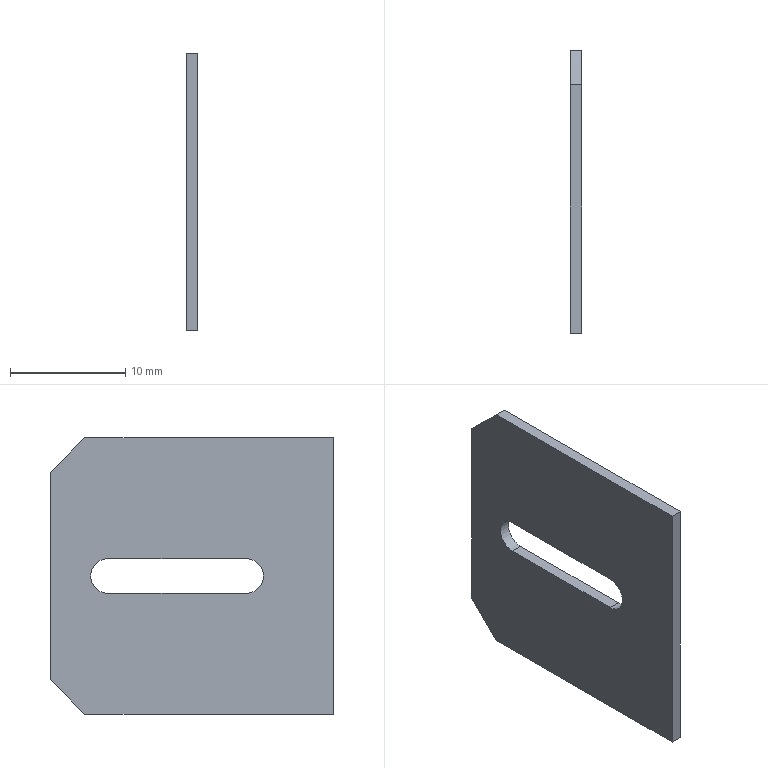Part | STEP file | ASND-0110-SDS_3_1 | 1 solid | 12 faces | box 1 x 24.6 x 24 mm | volume 538.331 mm3 | plane 10 | cylinder 2 | commonest cylinder face diameters 3 x2
STEP:
#1=CARTESIAN_POINT('',(0.,0.,0.));
#2=DIRECTION('',(0.,0.,1.));
#3=DIRECTION('',(1.,0.,0.));
#4=AXIS2_PLACEMENT_3D('',#1,#2,#3);
#5=CARTESIAN_POINT('',(-180.,82.3,67.4));
#6=VERTEX_POINT('',#5);
#7=CARTESIAN_POINT('',(-180.,79.3,70.4));
#8=VERTEX_POINT('',#7);
#9=CARTESIAN_POINT('',(-180.,82.3,67.4));
#10=DIRECTION('',(0.,-0.7071,0.7071));
#11=VECTOR('',#10,1.);
#12=LINE('',#9,#11);
#13=CARTESIAN_POINT('',(-180.5,80.8,68.9));
#14=DIRECTION('',(0.,0.7071,0.7071));
#15=DIRECTION('',(0.5774,-0.5774,0.5774));
#16=AXIS2_PLACEMENT_3D('',#13,#14,#15);
#17=PLANE('',#16);
#18=CARTESIAN_POINT('',(-1.443,1.633));
#19=DIRECTION('',(0.8165,-0.5774));
#20=VECTOR('',#19,1.);
#21=LINE('',#18,#20);
#22=(GEOMETRIC_REPRESENTATION_CONTEXT(2)PARAMETRIC_REPRESENTATION_CONTEXT()REPRESENTATION_CONTEXT('',''));
#23=DEFINITIONAL_REPRESENTATION('',(#21),#22);
#24=PCURVE('',#17,#23);
#25=CARTESIAN_POINT('',(-180.,0.,0.));
#26=DIRECTION('',(-1.,0.,0.));
#27=DIRECTION('',(0.,0.7071,0.7071));
#28=AXIS2_PLACEMENT_3D('',#25,#26,#27);
#29=PLANE('',#28);
#30=CARTESIAN_POINT('',(105.854,10.536));
#31=DIRECTION('',(0.,-1.));
#32=VECTOR('',#31,1.);
#33=LINE('',#30,#32);
#34=(GEOMETRIC_REPRESENTATION_CONTEXT(2)PARAMETRIC_REPRESENTATION_CONTEXT()REPRESENTATION_CONTEXT('',''));
#35=DEFINITIONAL_REPRESENTATION('',(#33),#34);
#36=PCURVE('',#29,#35);
#37=SURFACE_CURVE('',#12,(#24,#36),.PCURVE_S1.);
#38=EDGE_CURVE('',#6,#8,#37,.T.);
#39=ORIENTED_EDGE('',*,*,#38,.F.);
#40=CARTESIAN_POINT('',(-181.,82.3,67.4));
#41=VERTEX_POINT('',#40);
#42=CARTESIAN_POINT('',(-181.,82.3,67.4));
#43=DIRECTION('',(1.,0.,0.));
#44=VECTOR('',#43,1.);
#45=LINE('',#42,#44);
#46=CARTESIAN_POINT('',(-2.021,0.8165));
#47=DIRECTION('',(0.5774,0.8165));
#48=VECTOR('',#47,1.);
#49=LINE('',#46,#48);
#50=(GEOMETRIC_REPRESENTATION_CONTEXT(2)PARAMETRIC_REPRESENTATION_CONTEXT()REPRESENTATION_CONTEXT('',''));
#51=DEFINITIONAL_REPRESENTATION('',(#49),#50);
#52=PCURVE('',#17,#51);
#53=CARTESIAN_POINT('',(-181.,82.3,70.4));
#54=DIRECTION('',(0.,1.,0.));
#55=DIRECTION('',(0.7071,0.,0.7071));
#56=AXIS2_PLACEMENT_3D('',#53,#54,#55);
#57=PLANE('',#56);
#58=CARTESIAN_POINT('',(-2.121,2.121));
#59=DIRECTION('',(0.7071,0.7071));
#60=VECTOR('',#59,1.);
#61=LINE('',#58,#60);
#62=(GEOMETRIC_REPRESENTATION_CONTEXT(2)PARAMETRIC_REPRESENTATION_CONTEXT()REPRESENTATION_CONTEXT('',''));
#63=DEFINITIONAL_REPRESENTATION('',(#61),#62);
#64=PCURVE('',#57,#63);
#65=SURFACE_CURVE('',#45,(#52,#64),.PCURVE_S1.);
#66=EDGE_CURVE('',#41,#6,#65,.T.);
#67=ORIENTED_EDGE('',*,*,#66,.F.);
#68=CARTESIAN_POINT('',(-181.,79.3,70.4));
#69=VERTEX_POINT('',#68);
#70=CARTESIAN_POINT('',(-181.,79.3,70.4));
#71=DIRECTION('',(0.,0.7071,-0.7071));
#72=VECTOR('',#71,1.);
#73=LINE('',#70,#72);
#74=CARTESIAN_POINT('',(1.443,-1.633));
#75=DIRECTION('',(-0.8165,0.5774));
#76=VECTOR('',#75,1.);
#77=LINE('',#74,#76);
#78=(GEOMETRIC_REPRESENTATION_CONTEXT(2)PARAMETRIC_REPRESENTATION_CONTEXT()REPRESENTATION_CONTEXT('',''));
#79=DEFINITIONAL_REPRESENTATION('',(#77),#78);
#80=PCURVE('',#17,#79);
#81=CARTESIAN_POINT('',(-181.,0.,0.));
#82=DIRECTION('',(-1.,0.,0.));
#83=DIRECTION('',(0.,0.7071,0.7071));
#84=AXIS2_PLACEMENT_3D('',#81,#82,#83);
#85=PLANE('',#84);
#86=CARTESIAN_POINT('',(105.854,6.293));
#87=DIRECTION('',(0.,1.));
#88=VECTOR('',#87,1.);
#89=LINE('',#86,#88);
#90=(GEOMETRIC_REPRESENTATION_CONTEXT(2)PARAMETRIC_REPRESENTATION_CONTEXT()REPRESENTATION_CONTEXT('',''));
#91=DEFINITIONAL_REPRESENTATION('',(#89),#90);
#92=PCURVE('',#85,#91);
#93=SURFACE_CURVE('',#73,(#80,#92),.PCURVE_S1.);
#94=EDGE_CURVE('',#69,#41,#93,.T.);
#95=ORIENTED_EDGE('',*,*,#94,.F.);
#96=CARTESIAN_POINT('',(-181.,79.3,70.4));
#97=DIRECTION('',(1.,0.,0.));
#98=VECTOR('',#97,1.);
#99=LINE('',#96,#98);
#100=CARTESIAN_POINT('',(1.443,-1.633));
#101=DIRECTION('',(0.5774,0.8165));
#102=VECTOR('',#101,1.);
#103=LINE('',#100,#102);
#104=(GEOMETRIC_REPRESENTATION_CONTEXT(2)PARAMETRIC_REPRESENTATION_CONTEXT()REPRESENTATION_CONTEXT('',''));
#105=DEFINITIONAL_REPRESENTATION('',(#103),#104);
#106=PCURVE('',#17,#105);
#107=CARTESIAN_POINT('',(-181.,57.7,70.4));
#108=DIRECTION('',(0.,0.,1.));
#109=DIRECTION('',(0.7071,0.7071,0.));
#110=AXIS2_PLACEMENT_3D('',#107,#108,#109);
#111=PLANE('',#110);
#112=CARTESIAN_POINT('',(15.274,15.274));
#113=DIRECTION('',(0.7071,-0.7071));
#114=VECTOR('',#113,1.);
#115=LINE('',#112,#114);
#116=(GEOMETRIC_REPRESENTATION_CONTEXT(2)PARAMETRIC_REPRESENTATION_CONTEXT()REPRESENTATION_CONTEXT('',''));
#117=DEFINITIONAL_REPRESENTATION('',(#115),#116);
#118=PCURVE('',#111,#117);
#119=SURFACE_CURVE('',#99,(#106,#118),.PCURVE_S1.);
#120=EDGE_CURVE('',#69,#8,#119,.T.);
#121=ORIENTED_EDGE('',*,*,#120,.T.);
#122=EDGE_LOOP('',(#39,#67,#95,#121));
#123=FACE_BOUND('',#122,.T.);
#124=ADVANCED_FACE('',(#123),#17,.T.);
#125=CARTESIAN_POINT('',(-180.,79.3,46.4));
#126=VERTEX_POINT('',#125);
#127=CARTESIAN_POINT('',(-180.,82.3,49.4));
#128=VERTEX_POINT('',#127);
#129=CARTESIAN_POINT('',(-180.,79.3,46.4));
#130=DIRECTION('',(0.,0.7071,0.7071));
#131=VECTOR('',#130,1.);
#132=LINE('',#129,#131);
#133=CARTESIAN_POINT('',(88.883,23.264));
#134=DIRECTION('',(1.,0.));
#135=VECTOR('',#134,1.);
#136=LINE('',#133,#135);
#137=(GEOMETRIC_REPRESENTATION_CONTEXT(2)PARAMETRIC_REPRESENTATION_CONTEXT()REPRESENTATION_CONTEXT('',''));
#138=DEFINITIONAL_REPRESENTATION('',(#136),#137);
#139=PCURVE('',#29,#138);
#140=CARTESIAN_POINT('',(-180.5,80.8,47.9));
#141=DIRECTION('',(0.,0.7071,-0.7071));
#142=DIRECTION('',(0.5774,0.5774,0.5774));
#143=AXIS2_PLACEMENT_3D('',#140,#141,#142);
#144=PLANE('',#143);
#145=CARTESIAN_POINT('',(-1.443,1.633));
#146=DIRECTION('',(0.8165,-0.5774));
#147=VECTOR('',#146,1.);
#148=LINE('',#145,#147);
#149=(GEOMETRIC_REPRESENTATION_CONTEXT(2)PARAMETRIC_REPRESENTATION_CONTEXT()REPRESENTATION_CONTEXT('',''));
#150=DEFINITIONAL_REPRESENTATION('',(#148),#149);
#151=PCURVE('',#144,#150);
#152=SURFACE_CURVE('',#132,(#139,#151),.PCURVE_S1.);
#153=EDGE_CURVE('',#126,#128,#152,.T.);
#154=ORIENTED_EDGE('',*,*,#153,.T.);
#155=CARTESIAN_POINT('',(-180.,82.3,67.4));
#156=DIRECTION('',(0.,0.,-1.));
#157=VECTOR('',#156,1.);
#158=LINE('',#155,#157);
#159=CARTESIAN_POINT('',(105.854,10.536));
#160=DIRECTION('',(-0.7071,0.7071));
#161=VECTOR('',#160,1.);
#162=LINE('',#159,#161);
#163=(GEOMETRIC_REPRESENTATION_CONTEXT(2)PARAMETRIC_REPRESENTATION_CONTEXT()REPRESENTATION_CONTEXT('',''));
#164=DEFINITIONAL_REPRESENTATION('',(#162),#163);
#165=PCURVE('',#29,#164);
#166=CARTESIAN_POINT('',(-1.414,2.828));
#167=DIRECTION('',(-0.7071,0.7071));
#168=VECTOR('',#167,1.);
#169=LINE('',#166,#168);
#170=(GEOMETRIC_REPRESENTATION_CONTEXT(2)PARAMETRIC_REPRESENTATION_CONTEXT()REPRESENTATION_CONTEXT('',''));
#171=DEFINITIONAL_REPRESENTATION('',(#169),#170);
#172=PCURVE('',#57,#171);
#173=SURFACE_CURVE('',#158,(#165,#172),.PCURVE_S1.);
#174=EDGE_CURVE('',#6,#128,#173,.T.);
#175=ORIENTED_EDGE('',*,*,#174,.F.);
#176=ORIENTED_EDGE('',*,*,#38,.T.);
#177=CARTESIAN_POINT('',(-180.,57.7,70.4));
#178=VERTEX_POINT('',#177);
#179=CARTESIAN_POINT('',(-180.,57.7,70.4));
#180=DIRECTION('',(0.,1.,0.));
#181=VECTOR('',#180,1.);
#182=LINE('',#179,#181);
#183=CARTESIAN_POINT('',(90.58,-8.98));
#184=DIRECTION('',(0.7071,0.7071));
#185=VECTOR('',#184,1.);
#186=LINE('',#183,#185);
#187=(GEOMETRIC_REPRESENTATION_CONTEXT(2)PARAMETRIC_REPRESENTATION_CONTEXT()REPRESENTATION_CONTEXT('',''));
#188=DEFINITIONAL_REPRESENTATION('',(#186),#187);
#189=PCURVE('',#29,#188);
#190=CARTESIAN_POINT('',(0.7071,-0.7071));
#191=DIRECTION('',(0.7071,0.7071));
#192=VECTOR('',#191,1.);
#193=LINE('',#190,#192);
#194=(GEOMETRIC_REPRESENTATION_CONTEXT(2)PARAMETRIC_REPRESENTATION_CONTEXT()REPRESENTATION_CONTEXT('',''));
#195=DEFINITIONAL_REPRESENTATION('',(#193),#194);
#196=PCURVE('',#111,#195);
#197=SURFACE_CURVE('',#182,(#189,#196),.PCURVE_S1.);
#198=EDGE_CURVE('',#178,#8,#197,.T.);
#199=ORIENTED_EDGE('',*,*,#198,.F.);
#200=CARTESIAN_POINT('',(-180.,57.7,46.4));
#201=VERTEX_POINT('',#200);
#202=CARTESIAN_POINT('',(-180.,57.7,46.4));
#203=DIRECTION('',(0.,0.,1.));
#204=VECTOR('',#203,1.);
#205=LINE('',#202,#204);
#206=CARTESIAN_POINT('',(73.61,7.99));
#207=DIRECTION('',(0.7071,-0.7071));
#208=VECTOR('',#207,1.);
#209=LINE('',#206,#208);
#210=(GEOMETRIC_REPRESENTATION_CONTEXT(2)PARAMETRIC_REPRESENTATION_CONTEXT()REPRESENTATION_CONTEXT('',''));
#211=DEFINITIONAL_REPRESENTATION('',(#209),#210);
#212=PCURVE('',#29,#211);
#213=CARTESIAN_POINT('',(-181.,57.7,46.4));
#214=DIRECTION('',(0.,-1.,0.));
#215=DIRECTION('',(0.7071,0.,0.7071));
#216=AXIS2_PLACEMENT_3D('',#213,#214,#215);
#217=PLANE('',#216);
#218=CARTESIAN_POINT('',(0.7071,-0.7071));
#219=DIRECTION('',(0.7071,0.7071));
#220=VECTOR('',#219,1.);
#221=LINE('',#218,#220);
#222=(GEOMETRIC_REPRESENTATION_CONTEXT(2)PARAMETRIC_REPRESENTATION_CONTEXT()REPRESENTATION_CONTEXT('',''));
#223=DEFINITIONAL_REPRESENTATION('',(#221),#222);
#224=PCURVE('',#217,#223);
#225=SURFACE_CURVE('',#205,(#212,#224),.PCURVE_S1.);
#226=EDGE_CURVE('',#201,#178,#225,.T.);
#227=ORIENTED_EDGE('',*,*,#226,.F.);
#228=CARTESIAN_POINT('',(-180.,79.3,46.4));
#229=DIRECTION('',(0.,-1.,0.));
#230=VECTOR('',#229,1.);
#231=LINE('',#228,#230);
#232=CARTESIAN_POINT('',(88.883,23.264));
#233=DIRECTION('',(-0.7071,-0.7071));
#234=VECTOR('',#233,1.);
#235=LINE('',#232,#234);
#236=(GEOMETRIC_REPRESENTATION_CONTEXT(2)PARAMETRIC_REPRESENTATION_CONTEXT()REPRESENTATION_CONTEXT('',''));
#237=DEFINITIONAL_REPRESENTATION('',(#235),#236);
#238=PCURVE('',#29,#237);
#239=CARTESIAN_POINT('',(-181.,82.3,46.4));
#240=DIRECTION('',(0.,0.,-1.));
#241=DIRECTION('',(0.7071,0.7071,0.));
#242=AXIS2_PLACEMENT_3D('',#239,#240,#241);
#243=PLANE('',#242);
#244=CARTESIAN_POINT('',(-1.414,2.828));
#245=DIRECTION('',(-0.7071,0.7071));
#246=VECTOR('',#245,1.);
#247=LINE('',#244,#246);
#248=(GEOMETRIC_REPRESENTATION_CONTEXT(2)PARAMETRIC_REPRESENTATION_CONTEXT()REPRESENTATION_CONTEXT('',''));
#249=DEFINITIONAL_REPRESENTATION('',(#247),#248);
#250=PCURVE('',#243,#249);
#251=SURFACE_CURVE('',#231,(#238,#250),.PCURVE_S1.);
#252=EDGE_CURVE('',#126,#201,#251,.T.);
#253=ORIENTED_EDGE('',*,*,#252,.F.);
#254=EDGE_LOOP('',(#154,#175,#176,#199,#227,#253));
#255=FACE_BOUND('',#254,.T.);
#256=CARTESIAN_POINT('',(-180.,77.3,56.9));
#257=VERTEX_POINT('',#256);
#258=CARTESIAN_POINT('',(-180.,77.3,59.9));
#259=VERTEX_POINT('',#258);
#260=CARTESIAN_POINT('',(-180.,77.3,58.4));
#261=DIRECTION('',(1.,0.,0.));
#262=DIRECTION('',(0.,0.,-1.));
#263=AXIS2_PLACEMENT_3D('',#260,#261,#262);
#264=CIRCLE('',#263,1.5);
#265=CARTESIAN_POINT('',(94.894,14.425));
#266=CARTESIAN_POINT('',(96.731,16.262));
#267=CARTESIAN_POINT('',(97.403,13.753));
#268=CARTESIAN_POINT('',(98.076,11.243));
#269=CARTESIAN_POINT('',(95.566,11.915));
#270=CARTESIAN_POINT('',(93.057,12.588));
#271=CARTESIAN_POINT('',(94.894,14.425));
#272=(BOUNDED_CURVE()B_SPLINE_CURVE(2,(#265,#266,#267,#268,#269,#270,#271),.UNSPECIFIED.,.T.,.F.)B_SPLINE_CURVE_WITH_KNOTS((1,2,2,2,2,1),(-2.094,0.,2.094,4.189,6.283,8.378),.UNSPECIFIED.)CURVE()GEOMETRIC_REPRESENTATION_ITEM()RATIONAL_B_SPLINE_CURVE((1.,0.5,1.,0.5,1.,0.5,1.))REPRESENTATION_ITEM(''));
#273=(GEOMETRIC_REPRESENTATION_CONTEXT(2)PARAMETRIC_REPRESENTATION_CONTEXT()REPRESENTATION_CONTEXT('',''));
#274=DEFINITIONAL_REPRESENTATION('',(#272),#273);
#275=PCURVE('',#29,#274);
#276=CARTESIAN_POINT('',(-181.,77.3,58.4));
#277=DIRECTION('',(-1.,0.,0.));
#278=DIRECTION('',(0.,0.,1.));
#279=AXIS2_PLACEMENT_3D('',#276,#277,#278);
#280=CYLINDRICAL_SURFACE('',#279,1.5);
#281=CARTESIAN_POINT('',(3.142,-1.));
#282=DIRECTION('',(-1.,0.));
#283=VECTOR('',#282,1.);
#284=LINE('',#281,#283);
#285=(GEOMETRIC_REPRESENTATION_CONTEXT(2)PARAMETRIC_REPRESENTATION_CONTEXT()REPRESENTATION_CONTEXT('',''));
#286=DEFINITIONAL_REPRESENTATION('',(#284),#285);
#287=PCURVE('',#280,#286);
#288=SURFACE_CURVE('',#264,(#275,#287),.PCURVE_S1.);
#289=EDGE_CURVE('',#257,#259,#288,.T.);
#290=ORIENTED_EDGE('',*,*,#289,.F.);
#291=CARTESIAN_POINT('',(-180.,65.3,56.9));
#292=VERTEX_POINT('',#291);
#293=CARTESIAN_POINT('',(-180.,65.3,56.9));
#294=DIRECTION('',(0.,1.,0.));
#295=VECTOR('',#294,1.);
#296=LINE('',#293,#295);
#297=CARTESIAN_POINT('',(86.408,5.94));
#298=DIRECTION('',(0.7071,0.7071));
#299=VECTOR('',#298,1.);
#300=LINE('',#297,#299);
#301=(GEOMETRIC_REPRESENTATION_CONTEXT(2)PARAMETRIC_REPRESENTATION_CONTEXT()REPRESENTATION_CONTEXT('',''));
#302=DEFINITIONAL_REPRESENTATION('',(#300),#301);
#303=PCURVE('',#29,#302);
#304=CARTESIAN_POINT('',(-181.,65.3,56.9));
#305=DIRECTION('',(0.,0.,1.));
#306=DIRECTION('',(0.7071,0.7071,0.));
#307=AXIS2_PLACEMENT_3D('',#304,#305,#306);
#308=PLANE('',#307);
#309=CARTESIAN_POINT('',(0.7071,-0.7071));
#310=DIRECTION('',(0.7071,0.7071));
#311=VECTOR('',#310,1.);
#312=LINE('',#309,#311);
#313=(GEOMETRIC_REPRESENTATION_CONTEXT(2)PARAMETRIC_REPRESENTATION_CONTEXT()REPRESENTATION_CONTEXT('',''));
#314=DEFINITIONAL_REPRESENTATION('',(#312),#313);
#315=PCURVE('',#308,#314);
#316=SURFACE_CURVE('',#296,(#303,#315),.PCURVE_S1.);
#317=EDGE_CURVE('',#292,#257,#316,.T.);
#318=ORIENTED_EDGE('',*,*,#317,.F.);
#319=CARTESIAN_POINT('',(-180.,65.3,59.9));
#320=VERTEX_POINT('',#319);
#321=CARTESIAN_POINT('',(-180.,65.3,58.4));
#322=DIRECTION('',(1.,0.,0.));
#323=DIRECTION('',(0.,0.,1.));
#324=AXIS2_PLACEMENT_3D('',#321,#322,#323);
#325=CIRCLE('',#324,1.5);
#326=CARTESIAN_POINT('',(88.53,3.818));
#327=CARTESIAN_POINT('',(86.693,1.981));
#328=CARTESIAN_POINT('',(86.02,4.491));
#329=CARTESIAN_POINT('',(85.348,7.));
#330=CARTESIAN_POINT('',(87.857,6.328));
#331=CARTESIAN_POINT('',(90.367,5.655));
#332=CARTESIAN_POINT('',(88.53,3.818));
#333=(BOUNDED_CURVE()B_SPLINE_CURVE(2,(#326,#327,#328,#329,#330,#331,#332),.UNSPECIFIED.,.T.,.F.)B_SPLINE_CURVE_WITH_KNOTS((1,2,2,2,2,1),(-2.094,0.,2.094,4.189,6.283,8.378),.UNSPECIFIED.)CURVE()GEOMETRIC_REPRESENTATION_ITEM()RATIONAL_B_SPLINE_CURVE((1.,0.5,1.,0.5,1.,0.5,1.))REPRESENTATION_ITEM(''));
#334=(GEOMETRIC_REPRESENTATION_CONTEXT(2)PARAMETRIC_REPRESENTATION_CONTEXT()REPRESENTATION_CONTEXT('',''));
#335=DEFINITIONAL_REPRESENTATION('',(#333),#334);
#336=PCURVE('',#29,#335);
#337=CARTESIAN_POINT('',(-181.,65.3,58.4));
#338=DIRECTION('',(-1.,0.,0.));
#339=DIRECTION('',(0.,0.,1.));
#340=AXIS2_PLACEMENT_3D('',#337,#338,#339);
#341=CYLINDRICAL_SURFACE('',#340,1.5);
#342=CARTESIAN_POINT('',(6.283,-1.));
#343=DIRECTION('',(-1.,0.));
#344=VECTOR('',#343,1.);
#345=LINE('',#342,#344);
#346=(GEOMETRIC_REPRESENTATION_CONTEXT(2)PARAMETRIC_REPRESENTATION_CONTEXT()REPRESENTATION_CONTEXT('',''));
#347=DEFINITIONAL_REPRESENTATION('',(#345),#346);
#348=PCURVE('',#341,#347);
#349=SURFACE_CURVE('',#325,(#336,#348),.PCURVE_S1.);
#350=EDGE_CURVE('',#320,#292,#349,.T.);
#351=ORIENTED_EDGE('',*,*,#350,.F.);
#352=CARTESIAN_POINT('',(-180.,77.3,59.9));
#353=DIRECTION('',(0.,-1.,0.));
#354=VECTOR('',#353,1.);
#355=LINE('',#352,#354);
#356=CARTESIAN_POINT('',(97.015,12.304));
#357=DIRECTION('',(-0.7071,-0.7071));
#358=VECTOR('',#357,1.);
#359=LINE('',#356,#358);
#360=(GEOMETRIC_REPRESENTATION_CONTEXT(2)PARAMETRIC_REPRESENTATION_CONTEXT()REPRESENTATION_CONTEXT('',''));
#361=DEFINITIONAL_REPRESENTATION('',(#359),#360);
#362=PCURVE('',#29,#361);
#363=CARTESIAN_POINT('',(-181.,77.3,59.9));
#364=DIRECTION('',(0.,0.,-1.));
#365=DIRECTION('',(0.7071,0.7071,0.));
#366=AXIS2_PLACEMENT_3D('',#363,#364,#365);
#367=PLANE('',#366);
#368=CARTESIAN_POINT('',(0.7071,0.7071));
#369=DIRECTION('',(-0.7071,0.7071));
#370=VECTOR('',#369,1.);
#371=LINE('',#368,#370);
#372=(GEOMETRIC_REPRESENTATION_CONTEXT(2)PARAMETRIC_REPRESENTATION_CONTEXT()REPRESENTATION_CONTEXT('',''));
#373=DEFINITIONAL_REPRESENTATION('',(#371),#372);
#374=PCURVE('',#367,#373);
#375=SURFACE_CURVE('',#355,(#362,#374),.PCURVE_S1.);
#376=EDGE_CURVE('',#259,#320,#375,.T.);
#377=ORIENTED_EDGE('',*,*,#376,.F.);
#378=EDGE_LOOP('',(#290,#318,#351,#377));
#379=FACE_BOUND('',#378,.T.);
#380=ADVANCED_FACE('',(#255,#379),#29,.F.);
#381=CARTESIAN_POINT('',(-181.,77.3,59.9));
#382=VERTEX_POINT('',#381);
#383=CARTESIAN_POINT('',(-181.,77.3,59.9));
#384=DIRECTION('',(1.,0.,0.));
#385=VECTOR('',#384,1.);
#386=LINE('',#383,#385);
#387=CARTESIAN_POINT('',(0.,0.));
#388=DIRECTION('',(0.,-1.));
#389=VECTOR('',#388,1.);
#390=LINE('',#387,#389);
#391=(GEOMETRIC_REPRESENTATION_CONTEXT(2)PARAMETRIC_REPRESENTATION_CONTEXT()REPRESENTATION_CONTEXT('',''));
#392=DEFINITIONAL_REPRESENTATION('',(#390),#391);
#393=PCURVE('',#280,#392);
#394=CARTESIAN_POINT('',(0.,0.));
#395=DIRECTION('',(0.7071,0.7071));
#396=VECTOR('',#395,1.);
#397=LINE('',#394,#396);
#398=(GEOMETRIC_REPRESENTATION_CONTEXT(2)PARAMETRIC_REPRESENTATION_CONTEXT()REPRESENTATION_CONTEXT('',''));
#399=DEFINITIONAL_REPRESENTATION('',(#397),#398);
#400=PCURVE('',#367,#399);
#401=SURFACE_CURVE('',#386,(#393,#400),.PCURVE_S1.);
#402=EDGE_CURVE('',#382,#259,#401,.T.);
#403=ORIENTED_EDGE('',*,*,#402,.T.);
#404=ORIENTED_EDGE('',*,*,#289,.F.);
#405=CARTESIAN_POINT('',(-181.,77.3,56.9));
#406=VERTEX_POINT('',#405);
#407=CARTESIAN_POINT('',(-181.,77.3,56.9));
#408=DIRECTION('',(1.,0.,0.));
#409=VECTOR('',#408,1.);
#410=LINE('',#407,#409);
#411=CARTESIAN_POINT('',(3.142,0.));
#412=DIRECTION('',(0.,-1.));
#413=VECTOR('',#412,1.);
#414=LINE('',#411,#413);
#415=(GEOMETRIC_REPRESENTATION_CONTEXT(2)PARAMETRIC_REPRESENTATION_CONTEXT()REPRESENTATION_CONTEXT('',''));
#416=DEFINITIONAL_REPRESENTATION('',(#414),#415);
#417=PCURVE('',#280,#416);
#418=CARTESIAN_POINT('',(8.485,8.485));
#419=DIRECTION('',(0.7071,-0.7071));
#420=VECTOR('',#419,1.);
#421=LINE('',#418,#420);
#422=(GEOMETRIC_REPRESENTATION_CONTEXT(2)PARAMETRIC_REPRESENTATION_CONTEXT()REPRESENTATION_CONTEXT('',''));
#423=DEFINITIONAL_REPRESENTATION('',(#421),#422);
#424=PCURVE('',#308,#423);
#425=SURFACE_CURVE('',#410,(#417,#424),.PCURVE_S1.);
#426=EDGE_CURVE('',#406,#257,#425,.T.);
#427=ORIENTED_EDGE('',*,*,#426,.F.);
#428=CARTESIAN_POINT('',(-181.,77.3,58.4));
#429=DIRECTION('',(1.,0.,0.));
#430=DIRECTION('',(0.,0.,-1.));
#431=AXIS2_PLACEMENT_3D('',#428,#429,#430);
#432=CIRCLE('',#431,1.5);
#433=CARTESIAN_POINT('',(3.142,0.));
#434=DIRECTION('',(-1.,0.));
#435=VECTOR('',#434,1.);
#436=LINE('',#433,#435);
#437=(GEOMETRIC_REPRESENTATION_CONTEXT(2)PARAMETRIC_REPRESENTATION_CONTEXT()REPRESENTATION_CONTEXT('',''));
#438=DEFINITIONAL_REPRESENTATION('',(#436),#437);
#439=PCURVE('',#280,#438);
#440=CARTESIAN_POINT('',(94.894,14.425));
#441=CARTESIAN_POINT('',(96.731,16.262));
#442=CARTESIAN_POINT('',(97.403,13.753));
#443=CARTESIAN_POINT('',(98.076,11.243));
#444=CARTESIAN_POINT('',(95.566,11.915));
#445=CARTESIAN_POINT('',(93.057,12.588));
#446=CARTESIAN_POINT('',(94.894,14.425));
#447=(BOUNDED_CURVE()B_SPLINE_CURVE(2,(#440,#441,#442,#443,#444,#445,#446),.UNSPECIFIED.,.T.,.F.)B_SPLINE_CURVE_WITH_KNOTS((1,2,2,2,2,1),(-2.094,0.,2.094,4.189,6.283,8.378),.UNSPECIFIED.)CURVE()GEOMETRIC_REPRESENTATION_ITEM()RATIONAL_B_SPLINE_CURVE((1.,0.5,1.,0.5,1.,0.5,1.))REPRESENTATION_ITEM(''));
#448=(GEOMETRIC_REPRESENTATION_CONTEXT(2)PARAMETRIC_REPRESENTATION_CONTEXT()REPRESENTATION_CONTEXT('',''));
#449=DEFINITIONAL_REPRESENTATION('',(#447),#448);
#450=PCURVE('',#85,#449);
#451=SURFACE_CURVE('',#432,(#439,#450),.PCURVE_S1.);
#452=EDGE_CURVE('',#406,#382,#451,.T.);
#453=ORIENTED_EDGE('',*,*,#452,.T.);
#454=EDGE_LOOP('',(#403,#404,#427,#453));
#455=FACE_BOUND('',#454,.F.);
#456=ADVANCED_FACE('',(#455),#280,.F.);
#457=CARTESIAN_POINT('',(-181.,82.3,49.4));
#458=VERTEX_POINT('',#457);
#459=CARTESIAN_POINT('',(-181.,79.3,46.4));
#460=VERTEX_POINT('',#459);
#461=CARTESIAN_POINT('',(-181.,82.3,49.4));
#462=DIRECTION('',(0.,-0.7071,-0.7071));
#463=VECTOR('',#462,1.);
#464=LINE('',#461,#463);
#465=CARTESIAN_POINT('',(93.126,23.264));
#466=DIRECTION('',(-1.,0.));
#467=VECTOR('',#466,1.);
#468=LINE('',#465,#467);
#469=(GEOMETRIC_REPRESENTATION_CONTEXT(2)PARAMETRIC_REPRESENTATION_CONTEXT()REPRESENTATION_CONTEXT('',''));
#470=DEFINITIONAL_REPRESENTATION('',(#468),#469);
#471=PCURVE('',#85,#470);
#472=CARTESIAN_POINT('',(1.443,-1.633));
#473=DIRECTION('',(-0.8165,0.5774));
#474=VECTOR('',#473,1.);
#475=LINE('',#472,#474);
#476=(GEOMETRIC_REPRESENTATION_CONTEXT(2)PARAMETRIC_REPRESENTATION_CONTEXT()REPRESENTATION_CONTEXT('',''));
#477=DEFINITIONAL_REPRESENTATION('',(#475),#476);
#478=PCURVE('',#144,#477);
#479=SURFACE_CURVE('',#464,(#471,#478),.PCURVE_S1.);
#480=EDGE_CURVE('',#458,#460,#479,.T.);
#481=ORIENTED_EDGE('',*,*,#480,.T.);
#482=CARTESIAN_POINT('',(-181.,57.7,46.4));
#483=VERTEX_POINT('',#482);
#484=CARTESIAN_POINT('',(-181.,79.3,46.4));
#485=DIRECTION('',(0.,-1.,0.));
#486=VECTOR('',#485,1.);
#487=LINE('',#484,#486);
#488=CARTESIAN_POINT('',(88.883,23.264));
#489=DIRECTION('',(-0.7071,-0.7071));
#490=VECTOR('',#489,1.);
#491=LINE('',#488,#490);
#492=(GEOMETRIC_REPRESENTATION_CONTEXT(2)PARAMETRIC_REPRESENTATION_CONTEXT()REPRESENTATION_CONTEXT('',''));
#493=DEFINITIONAL_REPRESENTATION('',(#491),#492);
#494=PCURVE('',#85,#493);
#495=CARTESIAN_POINT('',(-2.121,2.121));
#496=DIRECTION('',(-0.7071,0.7071));
#497=VECTOR('',#496,1.);
#498=LINE('',#495,#497);
#499=(GEOMETRIC_REPRESENTATION_CONTEXT(2)PARAMETRIC_REPRESENTATION_CONTEXT()REPRESENTATION_CONTEXT('',''));
#500=DEFINITIONAL_REPRESENTATION('',(#498),#499);
#501=PCURVE('',#243,#500);
#502=SURFACE_CURVE('',#487,(#494,#501),.PCURVE_S1.);
#503=EDGE_CURVE('',#460,#483,#502,.T.);
#504=ORIENTED_EDGE('',*,*,#503,.T.);
#505=CARTESIAN_POINT('',(-181.,57.7,70.4));
#506=VERTEX_POINT('',#505);
#507=CARTESIAN_POINT('',(-181.,57.7,46.4));
#508=DIRECTION('',(0.,0.,1.));
#509=VECTOR('',#508,1.);
#510=LINE('',#507,#509);
#511=CARTESIAN_POINT('',(73.61,7.99));
#512=DIRECTION('',(0.7071,-0.7071));
#513=VECTOR('',#512,1.);
#514=LINE('',#511,#513);
#515=(GEOMETRIC_REPRESENTATION_CONTEXT(2)PARAMETRIC_REPRESENTATION_CONTEXT()REPRESENTATION_CONTEXT('',''));
#516=DEFINITIONAL_REPRESENTATION('',(#514),#515);
#517=PCURVE('',#85,#516);
#518=CARTESIAN_POINT('',(0.,0.));
#519=DIRECTION('',(0.7071,0.7071));
#520=VECTOR('',#519,1.);
#521=LINE('',#518,#520);
#522=(GEOMETRIC_REPRESENTATION_CONTEXT(2)PARAMETRIC_REPRESENTATION_CONTEXT()REPRESENTATION_CONTEXT('',''));
#523=DEFINITIONAL_REPRESENTATION('',(#521),#522);
#524=PCURVE('',#217,#523);
#525=SURFACE_CURVE('',#510,(#517,#524),.PCURVE_S1.);
#526=EDGE_CURVE('',#483,#506,#525,.T.);
#527=ORIENTED_EDGE('',*,*,#526,.T.);
#528=CARTESIAN_POINT('',(-181.,57.7,70.4));
#529=DIRECTION('',(0.,1.,0.));
#530=VECTOR('',#529,1.);
#531=LINE('',#528,#530);
#532=CARTESIAN_POINT('',(90.58,-8.98));
#533=DIRECTION('',(0.7071,0.7071));
#534=VECTOR('',#533,1.);
#535=LINE('',#532,#534);
#536=(GEOMETRIC_REPRESENTATION_CONTEXT(2)PARAMETRIC_REPRESENTATION_CONTEXT()REPRESENTATION_CONTEXT('',''));
#537=DEFINITIONAL_REPRESENTATION('',(#535),#536);
#538=PCURVE('',#85,#537);
#539=CARTESIAN_POINT('',(0.,0.));
#540=DIRECTION('',(0.7071,0.7071));
#541=VECTOR('',#540,1.);
#542=LINE('',#539,#541);
#543=(GEOMETRIC_REPRESENTATION_CONTEXT(2)PARAMETRIC_REPRESENTATION_CONTEXT()REPRESENTATION_CONTEXT('',''));
#544=DEFINITIONAL_REPRESENTATION('',(#542),#543);
#545=PCURVE('',#111,#544);
#546=SURFACE_CURVE('',#531,(#538,#545),.PCURVE_S1.);
#547=EDGE_CURVE('',#506,#69,#546,.T.);
#548=ORIENTED_EDGE('',*,*,#547,.T.);
#549=ORIENTED_EDGE('',*,*,#94,.T.);
#550=CARTESIAN_POINT('',(-181.,82.3,67.4));
#551=DIRECTION('',(0.,0.,-1.));
#552=VECTOR('',#551,1.);
#553=LINE('',#550,#552);
#554=CARTESIAN_POINT('',(105.854,10.536));
#555=DIRECTION('',(-0.7071,0.7071));
#556=VECTOR('',#555,1.);
#557=LINE('',#554,#556);
#558=(GEOMETRIC_REPRESENTATION_CONTEXT(2)PARAMETRIC_REPRESENTATION_CONTEXT()REPRESENTATION_CONTEXT('',''));
#559=DEFINITIONAL_REPRESENTATION('',(#557),#558);
#560=PCURVE('',#85,#559);
#561=CARTESIAN_POINT('',(-2.121,2.121));
#562=DIRECTION('',(-0.7071,0.7071));
#563=VECTOR('',#562,1.);
#564=LINE('',#561,#563);
#565=(GEOMETRIC_REPRESENTATION_CONTEXT(2)PARAMETRIC_REPRESENTATION_CONTEXT()REPRESENTATION_CONTEXT('',''));
#566=DEFINITIONAL_REPRESENTATION('',(#564),#565);
#567=PCURVE('',#57,#566);
#568=SURFACE_CURVE('',#553,(#560,#567),.PCURVE_S1.);
#569=EDGE_CURVE('',#41,#458,#568,.T.);
#570=ORIENTED_EDGE('',*,*,#569,.T.);
#571=EDGE_LOOP('',(#481,#504,#527,#548,#549,#570));
#572=FACE_BOUND('',#571,.T.);
#573=ORIENTED_EDGE('',*,*,#452,.T.);
#574=CARTESIAN_POINT('',(-181.,65.3,59.9));
#575=VERTEX_POINT('',#574);
#576=CARTESIAN_POINT('',(-181.,77.3,59.9));
#577=DIRECTION('',(0.,-1.,0.));
#578=VECTOR('',#577,1.);
#579=LINE('',#576,#578);
#580=CARTESIAN_POINT('',(97.015,12.304));
#581=DIRECTION('',(-0.7071,-0.7071));
#582=VECTOR('',#581,1.);
#583=LINE('',#580,#582);
#584=(GEOMETRIC_REPRESENTATION_CONTEXT(2)PARAMETRIC_REPRESENTATION_CONTEXT()REPRESENTATION_CONTEXT('',''));
#585=DEFINITIONAL_REPRESENTATION('',(#583),#584);
#586=PCURVE('',#85,#585);
#587=CARTESIAN_POINT('',(0.,0.));
#588=DIRECTION('',(-0.7071,0.7071));
#589=VECTOR('',#588,1.);
#590=LINE('',#587,#589);
#591=(GEOMETRIC_REPRESENTATION_CONTEXT(2)PARAMETRIC_REPRESENTATION_CONTEXT()REPRESENTATION_CONTEXT('',''));
#592=DEFINITIONAL_REPRESENTATION('',(#590),#591);
#593=PCURVE('',#367,#592);
#594=SURFACE_CURVE('',#579,(#586,#593),.PCURVE_S1.);
#595=EDGE_CURVE('',#382,#575,#594,.T.);
#596=ORIENTED_EDGE('',*,*,#595,.T.);
#597=CARTESIAN_POINT('',(-181.,65.3,56.9));
#598=VERTEX_POINT('',#597);
#599=CARTESIAN_POINT('',(-181.,65.3,58.4));
#600=DIRECTION('',(1.,0.,0.));
#601=DIRECTION('',(0.,0.,1.));
#602=AXIS2_PLACEMENT_3D('',#599,#600,#601);
#603=CIRCLE('',#602,1.5);
#604=CARTESIAN_POINT('',(88.53,3.818));
#605=CARTESIAN_POINT('',(86.693,1.981));
#606=CARTESIAN_POINT('',(86.02,4.491));
#607=CARTESIAN_POINT('',(85.348,7.));
#608=CARTESIAN_POINT('',(87.857,6.328));
#609=CARTESIAN_POINT('',(90.367,5.655));
#610=CARTESIAN_POINT('',(88.53,3.818));
#611=(BOUNDED_CURVE()B_SPLINE_CURVE(2,(#604,#605,#606,#607,#608,#609,#610),.UNSPECIFIED.,.T.,.F.)B_SPLINE_CURVE_WITH_KNOTS((1,2,2,2,2,1),(-2.094,0.,2.094,4.189,6.283,8.378),.UNSPECIFIED.)CURVE()GEOMETRIC_REPRESENTATION_ITEM()RATIONAL_B_SPLINE_CURVE((1.,0.5,1.,0.5,1.,0.5,1.))REPRESENTATION_ITEM(''));
#612=(GEOMETRIC_REPRESENTATION_CONTEXT(2)PARAMETRIC_REPRESENTATION_CONTEXT()REPRESENTATION_CONTEXT('',''));
#613=DEFINITIONAL_REPRESENTATION('',(#611),#612);
#614=PCURVE('',#85,#613);
#615=CARTESIAN_POINT('',(6.283,0.));
#616=DIRECTION('',(-1.,0.));
#617=VECTOR('',#616,1.);
#618=LINE('',#615,#617);
#619=(GEOMETRIC_REPRESENTATION_CONTEXT(2)PARAMETRIC_REPRESENTATION_CONTEXT()REPRESENTATION_CONTEXT('',''));
#620=DEFINITIONAL_REPRESENTATION('',(#618),#619);
#621=PCURVE('',#341,#620);
#622=SURFACE_CURVE('',#603,(#614,#621),.PCURVE_S1.);
#623=EDGE_CURVE('',#575,#598,#622,.T.);
#624=ORIENTED_EDGE('',*,*,#623,.T.);
#625=CARTESIAN_POINT('',(-181.,65.3,56.9));
#626=DIRECTION('',(0.,1.,0.));
#627=VECTOR('',#626,1.);
#628=LINE('',#625,#627);
#629=CARTESIAN_POINT('',(86.408,5.94));
#630=DIRECTION('',(0.7071,0.7071));
#631=VECTOR('',#630,1.);
#632=LINE('',#629,#631);
#633=(GEOMETRIC_REPRESENTATION_CONTEXT(2)PARAMETRIC_REPRESENTATION_CONTEXT()REPRESENTATION_CONTEXT('',''));
#634=DEFINITIONAL_REPRESENTATION('',(#632),#633);
#635=PCURVE('',#85,#634);
#636=CARTESIAN_POINT('',(0.,0.));
#637=DIRECTION('',(0.7071,0.7071));
#638=VECTOR('',#637,1.);
#639=LINE('',#636,#638);
#640=(GEOMETRIC_REPRESENTATION_CONTEXT(2)PARAMETRIC_REPRESENTATION_CONTEXT()REPRESENTATION_CONTEXT('',''));
#641=DEFINITIONAL_REPRESENTATION('',(#639),#640);
#642=PCURVE('',#308,#641);
#643=SURFACE_CURVE('',#628,(#635,#642),.PCURVE_S1.);
#644=EDGE_CURVE('',#598,#406,#643,.T.);
#645=ORIENTED_EDGE('',*,*,#644,.T.);
#646=EDGE_LOOP('',(#573,#596,#624,#645));
#647=FACE_BOUND('',#646,.T.);
#648=ADVANCED_FACE('',(#572,#647),#85,.T.);
#649=ORIENTED_EDGE('',*,*,#644,.F.);
#650=CARTESIAN_POINT('',(-181.,65.3,56.9));
#651=DIRECTION('',(1.,0.,0.));
#652=VECTOR('',#651,1.);
#653=LINE('',#650,#652);
#654=CARTESIAN_POINT('',(0.,0.));
#655=DIRECTION('',(0.7071,-0.7071));
#656=VECTOR('',#655,1.);
#657=LINE('',#654,#656);
#658=(GEOMETRIC_REPRESENTATION_CONTEXT(2)PARAMETRIC_REPRESENTATION_CONTEXT()REPRESENTATION_CONTEXT('',''));
#659=DEFINITIONAL_REPRESENTATION('',(#657),#658);
#660=PCURVE('',#308,#659);
#661=CARTESIAN_POINT('',(3.142,0.));
#662=DIRECTION('',(0.,-1.));
#663=VECTOR('',#662,1.);
#664=LINE('',#661,#663);
#665=(GEOMETRIC_REPRESENTATION_CONTEXT(2)PARAMETRIC_REPRESENTATION_CONTEXT()REPRESENTATION_CONTEXT('',''));
#666=DEFINITIONAL_REPRESENTATION('',(#664),#665);
#667=PCURVE('',#341,#666);
#668=SURFACE_CURVE('',#653,(#660,#667),.PCURVE_S1.);
#669=EDGE_CURVE('',#598,#292,#668,.T.);
#670=ORIENTED_EDGE('',*,*,#669,.T.);
#671=ORIENTED_EDGE('',*,*,#317,.T.);
#672=ORIENTED_EDGE('',*,*,#426,.F.);
#673=EDGE_LOOP('',(#649,#670,#671,#672));
#674=FACE_BOUND('',#673,.T.);
#675=ADVANCED_FACE('',(#674),#308,.T.);
#676=ORIENTED_EDGE('',*,*,#669,.T.);
#677=ORIENTED_EDGE('',*,*,#350,.F.);
#678=CARTESIAN_POINT('',(-181.,65.3,59.9));
#679=DIRECTION('',(1.,0.,0.));
#680=VECTOR('',#679,1.);
#681=LINE('',#678,#680);
#682=CARTESIAN_POINT('',(6.283,0.));
#683=DIRECTION('',(0.,-1.));
#684=VECTOR('',#683,1.);
#685=LINE('',#682,#684);
#686=(GEOMETRIC_REPRESENTATION_CONTEXT(2)PARAMETRIC_REPRESENTATION_CONTEXT()REPRESENTATION_CONTEXT('',''));
#687=DEFINITIONAL_REPRESENTATION('',(#685),#686);
#688=PCURVE('',#341,#687);
#689=CARTESIAN_POINT('',(-8.485,8.485));
#690=DIRECTION('',(0.7071,0.7071));
#691=VECTOR('',#690,1.);
#692=LINE('',#689,#691);
#693=(GEOMETRIC_REPRESENTATION_CONTEXT(2)PARAMETRIC_REPRESENTATION_CONTEXT()REPRESENTATION_CONTEXT('',''));
#694=DEFINITIONAL_REPRESENTATION('',(#692),#693);
#695=PCURVE('',#367,#694);
#696=SURFACE_CURVE('',#681,(#688,#695),.PCURVE_S1.);
#697=EDGE_CURVE('',#575,#320,#696,.T.);
#698=ORIENTED_EDGE('',*,*,#697,.F.);
#699=ORIENTED_EDGE('',*,*,#623,.T.);
#700=EDGE_LOOP('',(#676,#677,#698,#699));
#701=FACE_BOUND('',#700,.F.);
#702=ADVANCED_FACE('',(#701),#341,.F.);
#703=ORIENTED_EDGE('',*,*,#595,.F.);
#704=ORIENTED_EDGE('',*,*,#402,.T.);
#705=ORIENTED_EDGE('',*,*,#376,.T.);
#706=ORIENTED_EDGE('',*,*,#697,.F.);
#707=EDGE_LOOP('',(#703,#704,#705,#706));
#708=FACE_BOUND('',#707,.T.);
#709=ADVANCED_FACE('',(#708),#367,.T.);
#710=ORIENTED_EDGE('',*,*,#153,.F.);
#711=CARTESIAN_POINT('',(-181.,79.3,46.4));
#712=DIRECTION('',(1.,0.,0.));
#713=VECTOR('',#712,1.);
#714=LINE('',#711,#713);
#715=CARTESIAN_POINT('',(-2.021,0.8165));
#716=DIRECTION('',(0.5774,0.8165));
#717=VECTOR('',#716,1.);
#718=LINE('',#715,#717);
#719=(GEOMETRIC_REPRESENTATION_CONTEXT(2)PARAMETRIC_REPRESENTATION_CONTEXT()REPRESENTATION_CONTEXT('',''));
#720=DEFINITIONAL_REPRESENTATION('',(#718),#719);
#721=PCURVE('',#144,#720);
#722=CARTESIAN_POINT('',(-2.121,2.121));
#723=DIRECTION('',(0.7071,0.7071));
#724=VECTOR('',#723,1.);
#725=LINE('',#722,#724);
#726=(GEOMETRIC_REPRESENTATION_CONTEXT(2)PARAMETRIC_REPRESENTATION_CONTEXT()REPRESENTATION_CONTEXT('',''));
#727=DEFINITIONAL_REPRESENTATION('',(#725),#726);
#728=PCURVE('',#243,#727);
#729=SURFACE_CURVE('',#714,(#721,#728),.PCURVE_S1.);
#730=EDGE_CURVE('',#460,#126,#729,.T.);
#731=ORIENTED_EDGE('',*,*,#730,.F.);
#732=ORIENTED_EDGE('',*,*,#480,.F.);
#733=CARTESIAN_POINT('',(-181.,82.3,49.4));
#734=DIRECTION('',(1.,0.,0.));
#735=VECTOR('',#734,1.);
#736=LINE('',#733,#735);
#737=CARTESIAN_POINT('',(1.443,-1.633));
#738=DIRECTION('',(0.5774,0.8165));
#739=VECTOR('',#738,1.);
#740=LINE('',#737,#739);
#741=(GEOMETRIC_REPRESENTATION_CONTEXT(2)PARAMETRIC_REPRESENTATION_CONTEXT()REPRESENTATION_CONTEXT('',''));
#742=DEFINITIONAL_REPRESENTATION('',(#740),#741);
#743=PCURVE('',#144,#742);
#744=CARTESIAN_POINT('',(-14.849,14.849));
#745=DIRECTION('',(0.7071,0.7071));
#746=VECTOR('',#745,1.);
#747=LINE('',#744,#746);
#748=(GEOMETRIC_REPRESENTATION_CONTEXT(2)PARAMETRIC_REPRESENTATION_CONTEXT()REPRESENTATION_CONTEXT('',''));
#749=DEFINITIONAL_REPRESENTATION('',(#747),#748);
#750=PCURVE('',#57,#749);
#751=SURFACE_CURVE('',#736,(#743,#750),.PCURVE_S1.);
#752=EDGE_CURVE('',#458,#128,#751,.T.);
#753=ORIENTED_EDGE('',*,*,#752,.T.);
#754=EDGE_LOOP('',(#710,#731,#732,#753));
#755=FACE_BOUND('',#754,.T.);
#756=ADVANCED_FACE('',(#755),#144,.T.);
#757=ORIENTED_EDGE('',*,*,#752,.F.);
#758=ORIENTED_EDGE('',*,*,#569,.F.);
#759=ORIENTED_EDGE('',*,*,#66,.T.);
#760=ORIENTED_EDGE('',*,*,#174,.T.);
#761=EDGE_LOOP('',(#757,#758,#759,#760));
#762=FACE_BOUND('',#761,.T.);
#763=ADVANCED_FACE('',(#762),#57,.T.);
#764=ORIENTED_EDGE('',*,*,#730,.T.);
#765=ORIENTED_EDGE('',*,*,#252,.T.);
#766=CARTESIAN_POINT('',(-181.,57.7,46.4));
#767=DIRECTION('',(1.,0.,0.));
#768=VECTOR('',#767,1.);
#769=LINE('',#766,#768);
#770=CARTESIAN_POINT('',(-17.395,17.395));
#771=DIRECTION('',(0.7071,0.7071));
#772=VECTOR('',#771,1.);
#773=LINE('',#770,#772);
#774=(GEOMETRIC_REPRESENTATION_CONTEXT(2)PARAMETRIC_REPRESENTATION_CONTEXT()REPRESENTATION_CONTEXT('',''));
#775=DEFINITIONAL_REPRESENTATION('',(#773),#774);
#776=PCURVE('',#243,#775);
#777=CARTESIAN_POINT('',(0.,0.));
#778=DIRECTION('',(0.7071,-0.7071));
#779=VECTOR('',#778,1.);
#780=LINE('',#777,#779);
#781=(GEOMETRIC_REPRESENTATION_CONTEXT(2)PARAMETRIC_REPRESENTATION_CONTEXT()REPRESENTATION_CONTEXT('',''));
#782=DEFINITIONAL_REPRESENTATION('',(#780),#781);
#783=PCURVE('',#217,#782);
#784=SURFACE_CURVE('',#769,(#776,#783),.PCURVE_S1.);
#785=EDGE_CURVE('',#483,#201,#784,.T.);
#786=ORIENTED_EDGE('',*,*,#785,.F.);
#787=ORIENTED_EDGE('',*,*,#503,.F.);
#788=EDGE_LOOP('',(#764,#765,#786,#787));
#789=FACE_BOUND('',#788,.T.);
#790=ADVANCED_FACE('',(#789),#243,.T.);
#791=ORIENTED_EDGE('',*,*,#526,.F.);
#792=ORIENTED_EDGE('',*,*,#785,.T.);
#793=ORIENTED_EDGE('',*,*,#226,.T.);
#794=CARTESIAN_POINT('',(-181.,57.7,70.4));
#795=DIRECTION('',(1.,0.,0.));
#796=VECTOR('',#795,1.);
#797=LINE('',#794,#796);
#798=CARTESIAN_POINT('',(16.971,16.971));
#799=DIRECTION('',(0.7071,-0.7071));
#800=VECTOR('',#799,1.);
#801=LINE('',#798,#800);
#802=(GEOMETRIC_REPRESENTATION_CONTEXT(2)PARAMETRIC_REPRESENTATION_CONTEXT()REPRESENTATION_CONTEXT('',''));
#803=DEFINITIONAL_REPRESENTATION('',(#801),#802);
#804=PCURVE('',#217,#803);
#805=CARTESIAN_POINT('',(0.,0.));
#806=DIRECTION('',(0.7071,-0.7071));
#807=VECTOR('',#806,1.);
#808=LINE('',#805,#807);
#809=(GEOMETRIC_REPRESENTATION_CONTEXT(2)PARAMETRIC_REPRESENTATION_CONTEXT()REPRESENTATION_CONTEXT('',''));
#810=DEFINITIONAL_REPRESENTATION('',(#808),#809);
#811=PCURVE('',#111,#810);
#812=SURFACE_CURVE('',#797,(#804,#811),.PCURVE_S1.);
#813=EDGE_CURVE('',#506,#178,#812,.T.);
#814=ORIENTED_EDGE('',*,*,#813,.F.);
#815=EDGE_LOOP('',(#791,#792,#793,#814));
#816=FACE_BOUND('',#815,.T.);
#817=ADVANCED_FACE('',(#816),#217,.T.);
#818=ORIENTED_EDGE('',*,*,#120,.F.);
#819=ORIENTED_EDGE('',*,*,#547,.F.);
#820=ORIENTED_EDGE('',*,*,#813,.T.);
#821=ORIENTED_EDGE('',*,*,#198,.T.);
#822=EDGE_LOOP('',(#818,#819,#820,#821));
#823=FACE_BOUND('',#822,.T.);
#824=ADVANCED_FACE('',(#823),#111,.T.);
#825=CLOSED_SHELL('',(#124,#380,#456,#648,#675,#702,#709,#756,#763,#790,#817,#824));
#826=MANIFOLD_SOLID_BREP('',#825);
#827=(LENGTH_UNIT()NAMED_UNIT(*)SI_UNIT(.MILLI.,.METRE.));
#828=UNCERTAINTY_MEASURE_WITH_UNIT(LENGTH_MEASURE(0.0000001),#827,'','');
#829=(NAMED_UNIT(*)PLANE_ANGLE_UNIT()SI_UNIT($,.RADIAN.));
#830=(NAMED_UNIT(*)SI_UNIT($,.STERADIAN.)SOLID_ANGLE_UNIT());
#831=(GEOMETRIC_REPRESENTATION_CONTEXT(3)GLOBAL_UNCERTAINTY_ASSIGNED_CONTEXT((#828))GLOBAL_UNIT_ASSIGNED_CONTEXT((#827,#829,#830))REPRESENTATION_CONTEXT('',''));
#832=ADVANCED_BREP_SHAPE_REPRESENTATION('',(#4,#826),#831);